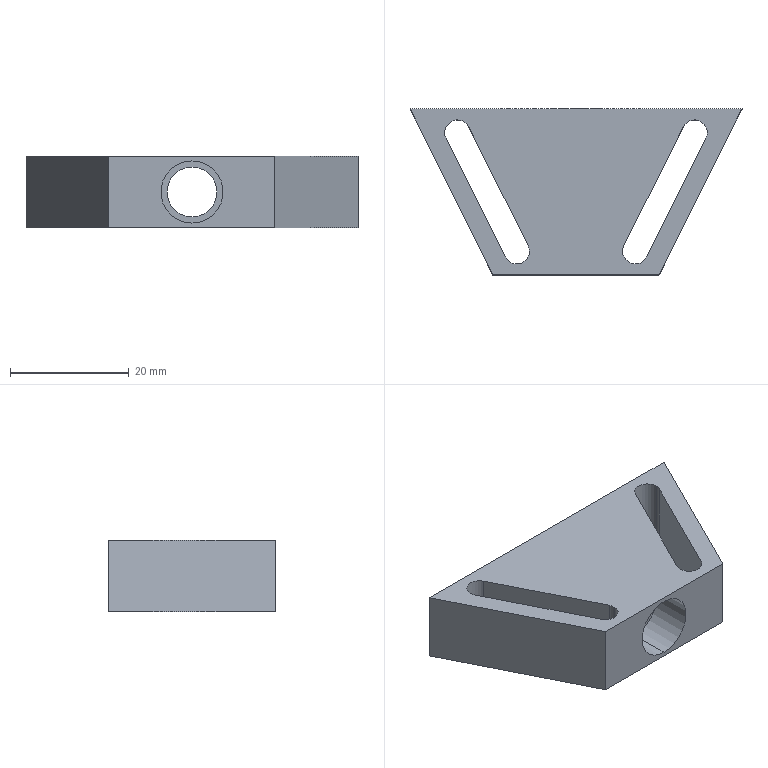Part | SolidWorks | features BaseBody 1 | 1 solid | 21 faces | box 56 x 28 x 12 mm | volume 9686 mm3 | plane 11 | cylinder 10 | commonest cylinder face diameters 4.3 x6 8.4 x2 10.5 x2
STEP:
#1=CARTESIAN_POINT('',(18.077,10.962,-6.));
#2=VERTEX_POINT('',#1);
#3=CARTESIAN_POINT('',(22.15,10.,-6.));
#4=VERTEX_POINT('',#3);
#5=CARTESIAN_POINT('',(20.,10.,-6.));
#6=DIRECTION('',(0.,0.,-1.));
#7=DIRECTION('',(1.,0.,0.));
#8=AXIS2_PLACEMENT_3D('',#5,#6,#7);
#9=CIRCLE('',#8,2.15);
#10=EDGE_CURVE('',#2,#4,#9,.T.);
#11=ORIENTED_EDGE('',*,*,#10,.T.);
#12=CARTESIAN_POINT('',(22.15,10.,6.));
#13=VERTEX_POINT('',#12);
#14=CARTESIAN_POINT('',(22.15,10.,-7.));
#15=DIRECTION('',(0.,0.,1.));
#16=VECTOR('',#15,1000.);
#17=LINE('',#14,#16);
#18=EDGE_CURVE('',#4,#13,#17,.T.);
#19=ORIENTED_EDGE('',*,*,#18,.T.);
#20=CARTESIAN_POINT('',(18.077,10.962,6.));
#21=VERTEX_POINT('',#20);
#22=CARTESIAN_POINT('',(20.,10.,6.));
#23=DIRECTION('',(0.,0.,-1.));
#24=DIRECTION('',(1.,0.,0.));
#25=AXIS2_PLACEMENT_3D('',#22,#23,#24);
#26=CIRCLE('',#25,2.15);
#27=EDGE_CURVE('',#21,#13,#26,.T.);
#28=ORIENTED_EDGE('',*,*,#27,.F.);
#29=CARTESIAN_POINT('',(18.077,10.962,-7.));
#30=DIRECTION('',(0.,0.,1.));
#31=VECTOR('',#30,1000.);
#32=LINE('',#29,#31);
#33=EDGE_CURVE('',#2,#21,#32,.T.);
#34=ORIENTED_EDGE('',*,*,#33,.F.);
#35=EDGE_LOOP('',(#11,#19,#28,#34));
#36=FACE_OUTER_BOUND('',#35,.T.);
#37=CARTESIAN_POINT('',(20.,10.,-7.));
#38=DIRECTION('',(0.,0.,1.));
#39=DIRECTION('',(1.,0.,0.));
#40=AXIS2_PLACEMENT_3D('',#37,#38,#39);
#41=CYLINDRICAL_SURFACE('',#40,2.15);
#42=ADVANCED_FACE('',(#36),#41,.F.);
#43=CARTESIAN_POINT('',(-8.077,-9.038,-6.));
#44=VERTEX_POINT('',#43);
#45=CARTESIAN_POINT('',(-7.85,-10.,-6.));
#46=VERTEX_POINT('',#45);
#47=CARTESIAN_POINT('',(-10.,-10.,-6.));
#48=DIRECTION('',(0.,0.,-1.));
#49=DIRECTION('',(1.,0.,0.));
#50=AXIS2_PLACEMENT_3D('',#47,#48,#49);
#51=CIRCLE('',#50,2.15);
#52=EDGE_CURVE('',#44,#46,#51,.T.);
#53=ORIENTED_EDGE('',*,*,#52,.T.);
#54=CARTESIAN_POINT('',(-7.85,-10.,6.));
#55=VERTEX_POINT('',#54);
#56=CARTESIAN_POINT('',(-7.85,-10.,-7.));
#57=DIRECTION('',(0.,0.,1.));
#58=VECTOR('',#57,1000.);
#59=LINE('',#56,#58);
#60=EDGE_CURVE('',#46,#55,#59,.T.);
#61=ORIENTED_EDGE('',*,*,#60,.T.);
#62=CARTESIAN_POINT('',(-8.077,-9.038,6.));
#63=VERTEX_POINT('',#62);
#64=CARTESIAN_POINT('',(-10.,-10.,6.));
#65=DIRECTION('',(0.,0.,-1.));
#66=DIRECTION('',(1.,0.,0.));
#67=AXIS2_PLACEMENT_3D('',#64,#65,#66);
#68=CIRCLE('',#67,2.15);
#69=EDGE_CURVE('',#63,#55,#68,.T.);
#70=ORIENTED_EDGE('',*,*,#69,.F.);
#71=CARTESIAN_POINT('',(-8.077,-9.038,-7.));
#72=DIRECTION('',(0.,0.,-1.));
#73=VECTOR('',#72,1000.);
#74=LINE('',#71,#73);
#75=EDGE_CURVE('',#63,#44,#74,.T.);
#76=ORIENTED_EDGE('',*,*,#75,.T.);
#77=EDGE_LOOP('',(#53,#61,#70,#76));
#78=FACE_OUTER_BOUND('',#77,.T.);
#79=CARTESIAN_POINT('',(-10.,-10.,-7.));
#80=DIRECTION('',(0.,0.,1.));
#81=DIRECTION('',(1.,0.,0.));
#82=AXIS2_PLACEMENT_3D('',#79,#80,#81);
#83=CYLINDRICAL_SURFACE('',#82,2.15);
#84=ADVANCED_FACE('',(#78),#83,.F.);
#85=CARTESIAN_POINT('',(0.,-7.,-4.2));
#86=VERTEX_POINT('',#85);
#87=CARTESIAN_POINT('',(0.,-7.,4.2));
#88=VERTEX_POINT('',#87);
#89=CARTESIAN_POINT('',(0.,-7.,0.));
#90=DIRECTION('',(0.,1.,0.));
#91=DIRECTION('',(0.,0.,1.));
#92=AXIS2_PLACEMENT_3D('',#89,#90,#91);
#93=CIRCLE('',#92,4.2);
#94=EDGE_CURVE('',#86,#88,#93,.T.);
#95=ORIENTED_EDGE('',*,*,#94,.F.);
#96=CARTESIAN_POINT('',(0.,14.,-4.2));
#97=VERTEX_POINT('',#96);
#98=CARTESIAN_POINT('',(0.,-16.,-4.2));
#99=DIRECTION('',(0.,1.,0.));
#100=VECTOR('',#99,1000.);
#101=LINE('',#98,#100);
#102=EDGE_CURVE('',#86,#97,#101,.T.);
#103=ORIENTED_EDGE('',*,*,#102,.T.);
#104=CARTESIAN_POINT('',(0.,14.,4.2));
#105=VERTEX_POINT('',#104);
#106=CARTESIAN_POINT('',(0.,14.,0.));
#107=DIRECTION('',(0.,1.,0.));
#108=DIRECTION('',(0.,0.,1.));
#109=AXIS2_PLACEMENT_3D('',#106,#107,#108);
#110=CIRCLE('',#109,4.2);
#111=EDGE_CURVE('',#97,#105,#110,.T.);
#112=ORIENTED_EDGE('',*,*,#111,.T.);
#113=CARTESIAN_POINT('',(0.,-16.,4.2));
#114=DIRECTION('',(0.,1.,0.));
#115=VECTOR('',#114,1000.);
#116=LINE('',#113,#115);
#117=EDGE_CURVE('',#88,#105,#116,.T.);
#118=ORIENTED_EDGE('',*,*,#117,.F.);
#119=EDGE_LOOP('',(#95,#103,#112,#118));
#120=FACE_OUTER_BOUND('',#119,.T.);
#121=CARTESIAN_POINT('',(0.,-16.,0.));
#122=DIRECTION('',(0.,1.,0.));
#123=DIRECTION('',(0.,0.,1.));
#124=AXIS2_PLACEMENT_3D('',#121,#122,#123);
#125=CYLINDRICAL_SURFACE('',#124,4.2);
#126=ADVANCED_FACE('',(#120),#125,.F.);
#127=CARTESIAN_POINT('',(0.,-14.,5.25));
#128=VERTEX_POINT('',#127);
#129=CARTESIAN_POINT('',(0.,-14.,-5.25));
#130=VERTEX_POINT('',#129);
#131=CARTESIAN_POINT('',(0.,-14.,0.));
#132=DIRECTION('',(0.,-1.,0.));
#133=DIRECTION('',(0.,0.,1.));
#134=AXIS2_PLACEMENT_3D('',#131,#132,#133);
#135=CIRCLE('',#134,5.25);
#136=EDGE_CURVE('',#128,#130,#135,.T.);
#137=ORIENTED_EDGE('',*,*,#136,.T.);
#138=CARTESIAN_POINT('',(0.,-7.,-5.25));
#139=VERTEX_POINT('',#138);
#140=CARTESIAN_POINT('',(0.,-14.,-5.25));
#141=DIRECTION('',(0.,1.,0.));
#142=VECTOR('',#141,1000.);
#143=LINE('',#140,#142);
#144=EDGE_CURVE('',#130,#139,#143,.T.);
#145=ORIENTED_EDGE('',*,*,#144,.T.);
#146=CARTESIAN_POINT('',(0.,-7.,5.25));
#147=VERTEX_POINT('',#146);
#148=CARTESIAN_POINT('',(0.,-7.,0.));
#149=DIRECTION('',(0.,-1.,0.));
#150=DIRECTION('',(0.,0.,1.));
#151=AXIS2_PLACEMENT_3D('',#148,#149,#150);
#152=CIRCLE('',#151,5.25);
#153=EDGE_CURVE('',#147,#139,#152,.T.);
#154=ORIENTED_EDGE('',*,*,#153,.F.);
#155=CARTESIAN_POINT('',(0.,-14.,5.25));
#156=DIRECTION('',(0.,1.,0.));
#157=VECTOR('',#156,1000.);
#158=LINE('',#155,#157);
#159=EDGE_CURVE('',#128,#147,#158,.T.);
#160=ORIENTED_EDGE('',*,*,#159,.F.);
#161=EDGE_LOOP('',(#137,#145,#154,#160));
#162=FACE_OUTER_BOUND('',#161,.T.);
#163=CARTESIAN_POINT('',(0.,-14.,0.));
#164=DIRECTION('',(0.,1.,0.));
#165=DIRECTION('',(0.,0.,1.));
#166=AXIS2_PLACEMENT_3D('',#163,#164,#165);
#167=CYLINDRICAL_SURFACE('',#166,5.25);
#168=ADVANCED_FACE('',(#162),#167,.F.);
#169=ORIENTED_EDGE('',*,*,#10,.F.);
#170=CARTESIAN_POINT('',(8.077,-9.038,-6.));
#171=VERTEX_POINT('',#170);
#172=CARTESIAN_POINT('',(8.077,-9.038,-6.));
#173=DIRECTION('',(0.4472,0.8944,0.));
#174=VECTOR('',#173,1000.);
#175=LINE('',#172,#174);
#176=EDGE_CURVE('',#171,#2,#175,.T.);
#177=ORIENTED_EDGE('',*,*,#176,.F.);
#178=CARTESIAN_POINT('',(11.923,-10.962,-6.));
#179=VERTEX_POINT('',#178);
#180=CARTESIAN_POINT('',(10.,-10.,-6.));
#181=DIRECTION('',(0.,0.,-1.));
#182=DIRECTION('',(1.,0.,0.));
#183=AXIS2_PLACEMENT_3D('',#180,#181,#182);
#184=CIRCLE('',#183,2.15);
#185=EDGE_CURVE('',#179,#171,#184,.T.);
#186=ORIENTED_EDGE('',*,*,#185,.F.);
#187=CARTESIAN_POINT('',(21.923,9.038,-6.));
#188=VERTEX_POINT('',#187);
#189=CARTESIAN_POINT('',(21.923,9.038,-6.));
#190=DIRECTION('',(-0.4472,-0.8944,0.));
#191=VECTOR('',#190,1000.);
#192=LINE('',#189,#191);
#193=EDGE_CURVE('',#188,#179,#192,.T.);
#194=ORIENTED_EDGE('',*,*,#193,.F.);
#195=CARTESIAN_POINT('',(20.,10.,-6.));
#196=DIRECTION('',(0.,0.,-1.));
#197=DIRECTION('',(1.,0.,0.));
#198=AXIS2_PLACEMENT_3D('',#195,#196,#197);
#199=CIRCLE('',#198,2.15);
#200=EDGE_CURVE('',#4,#188,#199,.T.);
#201=ORIENTED_EDGE('',*,*,#200,.F.);
#202=EDGE_LOOP('',(#169,#177,#186,#194,#201));
#203=FACE_BOUND('',#202,.T.);
#204=CARTESIAN_POINT('',(-21.923,9.038,-6.));
#205=VERTEX_POINT('',#204);
#206=CARTESIAN_POINT('',(-18.077,10.962,-6.));
#207=VERTEX_POINT('',#206);
#208=CARTESIAN_POINT('',(-20.,10.,-6.));
#209=DIRECTION('',(0.,0.,-1.));
#210=DIRECTION('',(1.,0.,0.));
#211=AXIS2_PLACEMENT_3D('',#208,#209,#210);
#212=CIRCLE('',#211,2.15);
#213=EDGE_CURVE('',#205,#207,#212,.T.);
#214=ORIENTED_EDGE('',*,*,#213,.F.);
#215=CARTESIAN_POINT('',(-11.923,-10.962,-6.));
#216=VERTEX_POINT('',#215);
#217=CARTESIAN_POINT('',(-11.923,-10.962,-6.));
#218=DIRECTION('',(-0.4472,0.8944,0.));
#219=VECTOR('',#218,1000.);
#220=LINE('',#217,#219);
#221=EDGE_CURVE('',#216,#205,#220,.T.);
#222=ORIENTED_EDGE('',*,*,#221,.F.);
#223=CARTESIAN_POINT('',(-10.,-10.,-6.));
#224=DIRECTION('',(0.,0.,-1.));
#225=DIRECTION('',(1.,0.,0.));
#226=AXIS2_PLACEMENT_3D('',#223,#224,#225);
#227=CIRCLE('',#226,2.15);
#228=EDGE_CURVE('',#46,#216,#227,.T.);
#229=ORIENTED_EDGE('',*,*,#228,.F.);
#230=ORIENTED_EDGE('',*,*,#52,.F.);
#231=CARTESIAN_POINT('',(-18.077,10.962,-6.));
#232=DIRECTION('',(0.4472,-0.8944,0.));
#233=VECTOR('',#232,1000.);
#234=LINE('',#231,#233);
#235=EDGE_CURVE('',#207,#44,#234,.T.);
#236=ORIENTED_EDGE('',*,*,#235,.F.);
#237=EDGE_LOOP('',(#214,#222,#229,#230,#236));
#238=FACE_BOUND('',#237,.T.);
#239=CARTESIAN_POINT('',(28.,14.,-6.));
#240=VERTEX_POINT('',#239);
#241=CARTESIAN_POINT('',(-28.,14.,-6.));
#242=VERTEX_POINT('',#241);
#243=CARTESIAN_POINT('',(0.,14.,-6.));
#244=DIRECTION('',(-1.,0.,0.));
#245=VECTOR('',#244,1000.);
#246=LINE('',#243,#245);
#247=EDGE_CURVE('',#240,#242,#246,.T.);
#248=ORIENTED_EDGE('',*,*,#247,.F.);
#249=CARTESIAN_POINT('',(14.,-14.,-6.));
#250=VERTEX_POINT('',#249);
#251=CARTESIAN_POINT('',(14.,-14.,-6.));
#252=DIRECTION('',(0.4472,0.8944,0.));
#253=VECTOR('',#252,1000.);
#254=LINE('',#251,#253);
#255=EDGE_CURVE('',#250,#240,#254,.T.);
#256=ORIENTED_EDGE('',*,*,#255,.F.);
#257=CARTESIAN_POINT('',(-14.,-14.,-6.));
#258=VERTEX_POINT('',#257);
#259=CARTESIAN_POINT('',(0.,-14.,-6.));
#260=DIRECTION('',(1.,0.,0.));
#261=VECTOR('',#260,1000.);
#262=LINE('',#259,#261);
#263=EDGE_CURVE('',#258,#250,#262,.T.);
#264=ORIENTED_EDGE('',*,*,#263,.F.);
#265=CARTESIAN_POINT('',(-28.,14.,-6.));
#266=DIRECTION('',(0.4472,-0.8944,0.));
#267=VECTOR('',#266,1000.);
#268=LINE('',#265,#267);
#269=EDGE_CURVE('',#242,#258,#268,.T.);
#270=ORIENTED_EDGE('',*,*,#269,.F.);
#271=EDGE_LOOP('',(#248,#256,#264,#270));
#272=FACE_OUTER_BOUND('',#271,.T.);
#273=CARTESIAN_POINT('',(0.,2.674,-6.));
#274=DIRECTION('',(0.,0.,1.));
#275=DIRECTION('',(1.,0.,0.));
#276=AXIS2_PLACEMENT_3D('',#273,#274,#275);
#277=PLANE('',#276);
#278=ADVANCED_FACE('',(#203,#238,#272),#277,.F.);
#279=CARTESIAN_POINT('',(21.923,9.038,6.));
#280=VERTEX_POINT('',#279);
#281=CARTESIAN_POINT('',(21.923,9.038,-7.));
#282=DIRECTION('',(0.,0.,1.));
#283=VECTOR('',#282,1000.);
#284=LINE('',#281,#283);
#285=EDGE_CURVE('',#188,#280,#284,.T.);
#286=ORIENTED_EDGE('',*,*,#285,.F.);
#287=ORIENTED_EDGE('',*,*,#193,.T.);
#288=CARTESIAN_POINT('',(11.923,-10.962,6.));
#289=VERTEX_POINT('',#288);
#290=CARTESIAN_POINT('',(11.923,-10.962,-7.));
#291=DIRECTION('',(0.,0.,-1.));
#292=VECTOR('',#291,1000.);
#293=LINE('',#290,#292);
#294=EDGE_CURVE('',#289,#179,#293,.T.);
#295=ORIENTED_EDGE('',*,*,#294,.F.);
#296=CARTESIAN_POINT('',(11.923,-10.962,6.));
#297=DIRECTION('',(-0.4472,-0.8944,0.));
#298=VECTOR('',#297,1000.);
#299=LINE('',#296,#298);
#300=EDGE_CURVE('',#280,#289,#299,.T.);
#301=ORIENTED_EDGE('',*,*,#300,.F.);
#302=EDGE_LOOP('',(#286,#287,#295,#301));
#303=FACE_OUTER_BOUND('',#302,.T.);
#304=CARTESIAN_POINT('',(11.923,-10.962,-7.));
#305=DIRECTION('',(0.8944,-0.4472,0.));
#306=DIRECTION('',(0.4472,0.8944,0.));
#307=AXIS2_PLACEMENT_3D('',#304,#305,#306);
#308=PLANE('',#307);
#309=ADVANCED_FACE('',(#303),#308,.F.);
#310=ORIENTED_EDGE('',*,*,#18,.F.);
#311=ORIENTED_EDGE('',*,*,#200,.T.);
#312=ORIENTED_EDGE('',*,*,#285,.T.);
#313=CARTESIAN_POINT('',(20.,10.,6.));
#314=DIRECTION('',(0.,0.,-1.));
#315=DIRECTION('',(1.,0.,0.));
#316=AXIS2_PLACEMENT_3D('',#313,#314,#315);
#317=CIRCLE('',#316,2.15);
#318=EDGE_CURVE('',#13,#280,#317,.T.);
#319=ORIENTED_EDGE('',*,*,#318,.F.);
#320=EDGE_LOOP('',(#310,#311,#312,#319));
#321=FACE_OUTER_BOUND('',#320,.T.);
#322=CARTESIAN_POINT('',(20.,10.,-7.));
#323=DIRECTION('',(0.,0.,1.));
#324=DIRECTION('',(1.,0.,0.));
#325=AXIS2_PLACEMENT_3D('',#322,#323,#324);
#326=CYLINDRICAL_SURFACE('',#325,2.15);
#327=ADVANCED_FACE('',(#321),#326,.F.);
#328=ORIENTED_EDGE('',*,*,#33,.T.);
#329=CARTESIAN_POINT('',(8.077,-9.038,6.));
#330=VERTEX_POINT('',#329);
#331=CARTESIAN_POINT('',(8.077,-9.038,6.));
#332=DIRECTION('',(-0.4472,-0.8944,0.));
#333=VECTOR('',#332,1000.);
#334=LINE('',#331,#333);
#335=EDGE_CURVE('',#21,#330,#334,.T.);
#336=ORIENTED_EDGE('',*,*,#335,.T.);
#337=CARTESIAN_POINT('',(8.077,-9.038,-7.));
#338=DIRECTION('',(0.,0.,-1.));
#339=VECTOR('',#338,1000.);
#340=LINE('',#337,#339);
#341=EDGE_CURVE('',#330,#171,#340,.T.);
#342=ORIENTED_EDGE('',*,*,#341,.T.);
#343=ORIENTED_EDGE('',*,*,#176,.T.);
#344=EDGE_LOOP('',(#328,#336,#342,#343));
#345=FACE_OUTER_BOUND('',#344,.T.);
#346=CARTESIAN_POINT('',(8.077,-9.038,-7.));
#347=DIRECTION('',(0.8944,-0.4472,0.));
#348=DIRECTION('',(0.4472,0.8944,0.));
#349=AXIS2_PLACEMENT_3D('',#346,#347,#348);
#350=PLANE('',#349);
#351=ADVANCED_FACE('',(#345),#350,.T.);
#352=ORIENTED_EDGE('',*,*,#185,.T.);
#353=ORIENTED_EDGE('',*,*,#341,.F.);
#354=CARTESIAN_POINT('',(10.,-10.,6.));
#355=DIRECTION('',(0.,0.,-1.));
#356=DIRECTION('',(1.,0.,0.));
#357=AXIS2_PLACEMENT_3D('',#354,#355,#356);
#358=CIRCLE('',#357,2.15);
#359=EDGE_CURVE('',#289,#330,#358,.T.);
#360=ORIENTED_EDGE('',*,*,#359,.F.);
#361=ORIENTED_EDGE('',*,*,#294,.T.);
#362=EDGE_LOOP('',(#352,#353,#360,#361));
#363=FACE_OUTER_BOUND('',#362,.T.);
#364=CARTESIAN_POINT('',(10.,-10.,-7.));
#365=DIRECTION('',(0.,0.,1.));
#366=DIRECTION('',(1.,0.,0.));
#367=AXIS2_PLACEMENT_3D('',#364,#365,#366);
#368=CYLINDRICAL_SURFACE('',#367,2.15);
#369=ADVANCED_FACE('',(#363),#368,.F.);
#370=CARTESIAN_POINT('',(-18.077,10.962,6.));
#371=VERTEX_POINT('',#370);
#372=CARTESIAN_POINT('',(-18.077,10.962,-7.));
#373=DIRECTION('',(0.,0.,1.));
#374=VECTOR('',#373,1000.);
#375=LINE('',#372,#374);
#376=EDGE_CURVE('',#207,#371,#375,.T.);
#377=ORIENTED_EDGE('',*,*,#376,.F.);
#378=ORIENTED_EDGE('',*,*,#235,.T.);
#379=ORIENTED_EDGE('',*,*,#75,.F.);
#380=CARTESIAN_POINT('',(-8.077,-9.038,6.));
#381=DIRECTION('',(0.4472,-0.8944,0.));
#382=VECTOR('',#381,1000.);
#383=LINE('',#380,#382);
#384=EDGE_CURVE('',#371,#63,#383,.T.);
#385=ORIENTED_EDGE('',*,*,#384,.F.);
#386=EDGE_LOOP('',(#377,#378,#379,#385));
#387=FACE_OUTER_BOUND('',#386,.T.);
#388=CARTESIAN_POINT('',(-8.077,-9.038,-7.));
#389=DIRECTION('',(0.8944,0.4472,0.));
#390=DIRECTION('',(-0.4472,0.8944,0.));
#391=AXIS2_PLACEMENT_3D('',#388,#389,#390);
#392=PLANE('',#391);
#393=ADVANCED_FACE('',(#387),#392,.F.);
#394=ORIENTED_EDGE('',*,*,#213,.T.);
#395=ORIENTED_EDGE('',*,*,#376,.T.);
#396=CARTESIAN_POINT('',(-21.923,9.038,6.));
#397=VERTEX_POINT('',#396);
#398=CARTESIAN_POINT('',(-20.,10.,6.));
#399=DIRECTION('',(0.,0.,-1.));
#400=DIRECTION('',(1.,0.,0.));
#401=AXIS2_PLACEMENT_3D('',#398,#399,#400);
#402=CIRCLE('',#401,2.15);
#403=EDGE_CURVE('',#397,#371,#402,.T.);
#404=ORIENTED_EDGE('',*,*,#403,.F.);
#405=CARTESIAN_POINT('',(-21.923,9.038,-7.));
#406=DIRECTION('',(0.,0.,1.));
#407=VECTOR('',#406,1000.);
#408=LINE('',#405,#407);
#409=EDGE_CURVE('',#205,#397,#408,.T.);
#410=ORIENTED_EDGE('',*,*,#409,.F.);
#411=EDGE_LOOP('',(#394,#395,#404,#410));
#412=FACE_OUTER_BOUND('',#411,.T.);
#413=CARTESIAN_POINT('',(-20.,10.,-7.));
#414=DIRECTION('',(0.,0.,1.));
#415=DIRECTION('',(1.,0.,0.));
#416=AXIS2_PLACEMENT_3D('',#413,#414,#415);
#417=CYLINDRICAL_SURFACE('',#416,2.15);
#418=ADVANCED_FACE('',(#412),#417,.F.);
#419=ORIENTED_EDGE('',*,*,#409,.T.);
#420=CARTESIAN_POINT('',(-11.923,-10.962,6.));
#421=VERTEX_POINT('',#420);
#422=CARTESIAN_POINT('',(-11.923,-10.962,6.));
#423=DIRECTION('',(0.4472,-0.8944,0.));
#424=VECTOR('',#423,1000.);
#425=LINE('',#422,#424);
#426=EDGE_CURVE('',#397,#421,#425,.T.);
#427=ORIENTED_EDGE('',*,*,#426,.T.);
#428=CARTESIAN_POINT('',(-11.923,-10.962,-7.));
#429=DIRECTION('',(0.,0.,-1.));
#430=VECTOR('',#429,1000.);
#431=LINE('',#428,#430);
#432=EDGE_CURVE('',#421,#216,#431,.T.);
#433=ORIENTED_EDGE('',*,*,#432,.T.);
#434=ORIENTED_EDGE('',*,*,#221,.T.);
#435=EDGE_LOOP('',(#419,#427,#433,#434));
#436=FACE_OUTER_BOUND('',#435,.T.);
#437=CARTESIAN_POINT('',(-11.923,-10.962,-7.));
#438=DIRECTION('',(0.8944,0.4472,0.));
#439=DIRECTION('',(-0.4472,0.8944,0.));
#440=AXIS2_PLACEMENT_3D('',#437,#438,#439);
#441=PLANE('',#440);
#442=ADVANCED_FACE('',(#436),#441,.T.);
#443=ORIENTED_EDGE('',*,*,#60,.F.);
#444=ORIENTED_EDGE('',*,*,#228,.T.);
#445=ORIENTED_EDGE('',*,*,#432,.F.);
#446=CARTESIAN_POINT('',(-10.,-10.,6.));
#447=DIRECTION('',(0.,0.,-1.));
#448=DIRECTION('',(1.,0.,0.));
#449=AXIS2_PLACEMENT_3D('',#446,#447,#448);
#450=CIRCLE('',#449,2.15);
#451=EDGE_CURVE('',#55,#421,#450,.T.);
#452=ORIENTED_EDGE('',*,*,#451,.F.);
#453=EDGE_LOOP('',(#443,#444,#445,#452));
#454=FACE_OUTER_BOUND('',#453,.T.);
#455=CARTESIAN_POINT('',(-10.,-10.,-7.));
#456=DIRECTION('',(0.,0.,1.));
#457=DIRECTION('',(1.,0.,0.));
#458=AXIS2_PLACEMENT_3D('',#455,#456,#457);
#459=CYLINDRICAL_SURFACE('',#458,2.15);
#460=ADVANCED_FACE('',(#454),#459,.F.);
#461=CARTESIAN_POINT('',(-14.,-14.,6.));
#462=VERTEX_POINT('',#461);
#463=CARTESIAN_POINT('',(-14.,-14.,-6.));
#464=DIRECTION('',(0.,0.,-1.));
#465=VECTOR('',#464,1000.);
#466=LINE('',#463,#465);
#467=EDGE_CURVE('',#462,#258,#466,.T.);
#468=ORIENTED_EDGE('',*,*,#467,.F.);
#469=CARTESIAN_POINT('',(-28.,14.,6.));
#470=VERTEX_POINT('',#469);
#471=CARTESIAN_POINT('',(-28.,14.,6.));
#472=DIRECTION('',(0.4472,-0.8944,0.));
#473=VECTOR('',#472,1000.);
#474=LINE('',#471,#473);
#475=EDGE_CURVE('',#470,#462,#474,.T.);
#476=ORIENTED_EDGE('',*,*,#475,.F.);
#477=CARTESIAN_POINT('',(-28.,14.,-6.));
#478=DIRECTION('',(0.,0.,1.));
#479=VECTOR('',#478,1000.);
#480=LINE('',#477,#479);
#481=EDGE_CURVE('',#242,#470,#480,.T.);
#482=ORIENTED_EDGE('',*,*,#481,.F.);
#483=ORIENTED_EDGE('',*,*,#269,.T.);
#484=EDGE_LOOP('',(#468,#476,#482,#483));
#485=FACE_OUTER_BOUND('',#484,.T.);
#486=CARTESIAN_POINT('',(-28.,14.,-6.));
#487=DIRECTION('',(0.8944,0.4472,0.));
#488=DIRECTION('',(-0.4472,0.8944,0.));
#489=AXIS2_PLACEMENT_3D('',#486,#487,#488);
#490=PLANE('',#489);
#491=ADVANCED_FACE('',(#485),#490,.F.);
#492=CARTESIAN_POINT('',(0.,14.,0.));
#493=DIRECTION('',(0.,1.,0.));
#494=DIRECTION('',(0.,0.,1.));
#495=AXIS2_PLACEMENT_3D('',#492,#493,#494);
#496=CIRCLE('',#495,4.2);
#497=EDGE_CURVE('',#105,#97,#496,.T.);
#498=ORIENTED_EDGE('',*,*,#497,.F.);
#499=ORIENTED_EDGE('',*,*,#111,.F.);
#500=EDGE_LOOP('',(#498,#499));
#501=FACE_BOUND('',#500,.T.);
#502=ORIENTED_EDGE('',*,*,#481,.T.);
#503=CARTESIAN_POINT('',(28.,14.,6.));
#504=VERTEX_POINT('',#503);
#505=CARTESIAN_POINT('',(28.,14.,6.));
#506=DIRECTION('',(-1.,0.,0.));
#507=VECTOR('',#506,1000.);
#508=LINE('',#505,#507);
#509=EDGE_CURVE('',#504,#470,#508,.T.);
#510=ORIENTED_EDGE('',*,*,#509,.F.);
#511=CARTESIAN_POINT('',(28.,14.,-6.));
#512=DIRECTION('',(0.,0.,1.));
#513=VECTOR('',#512,1000.);
#514=LINE('',#511,#513);
#515=EDGE_CURVE('',#240,#504,#514,.T.);
#516=ORIENTED_EDGE('',*,*,#515,.F.);
#517=ORIENTED_EDGE('',*,*,#247,.T.);
#518=EDGE_LOOP('',(#502,#510,#516,#517));
#519=FACE_OUTER_BOUND('',#518,.T.);
#520=CARTESIAN_POINT('',(28.,14.,-6.));
#521=DIRECTION('',(0.,-1.,0.));
#522=DIRECTION('',(0.,0.,-1.));
#523=AXIS2_PLACEMENT_3D('',#520,#521,#522);
#524=PLANE('',#523);
#525=ADVANCED_FACE('',(#501,#519),#524,.F.);
#526=ORIENTED_EDGE('',*,*,#515,.T.);
#527=CARTESIAN_POINT('',(14.,-14.,6.));
#528=VERTEX_POINT('',#527);
#529=CARTESIAN_POINT('',(14.,-14.,6.));
#530=DIRECTION('',(0.4472,0.8944,0.));
#531=VECTOR('',#530,1000.);
#532=LINE('',#529,#531);
#533=EDGE_CURVE('',#528,#504,#532,.T.);
#534=ORIENTED_EDGE('',*,*,#533,.F.);
#535=CARTESIAN_POINT('',(14.,-14.,-6.));
#536=DIRECTION('',(0.,0.,1.));
#537=VECTOR('',#536,1000.);
#538=LINE('',#535,#537);
#539=EDGE_CURVE('',#250,#528,#538,.T.);
#540=ORIENTED_EDGE('',*,*,#539,.F.);
#541=ORIENTED_EDGE('',*,*,#255,.T.);
#542=EDGE_LOOP('',(#526,#534,#540,#541));
#543=FACE_OUTER_BOUND('',#542,.T.);
#544=CARTESIAN_POINT('',(14.,-14.,-6.));
#545=DIRECTION('',(-0.8944,0.4472,0.));
#546=DIRECTION('',(-0.4472,-0.8944,0.));
#547=AXIS2_PLACEMENT_3D('',#544,#545,#546);
#548=PLANE('',#547);
#549=ADVANCED_FACE('',(#543),#548,.F.);
#550=ORIENTED_EDGE('',*,*,#136,.F.);
#551=CARTESIAN_POINT('',(0.,-14.,0.));
#552=DIRECTION('',(0.,-1.,0.));
#553=DIRECTION('',(0.,0.,1.));
#554=AXIS2_PLACEMENT_3D('',#551,#552,#553);
#555=CIRCLE('',#554,5.25);
#556=EDGE_CURVE('',#130,#128,#555,.T.);
#557=ORIENTED_EDGE('',*,*,#556,.F.);
#558=EDGE_LOOP('',(#550,#557));
#559=FACE_BOUND('',#558,.T.);
#560=ORIENTED_EDGE('',*,*,#539,.T.);
#561=CARTESIAN_POINT('',(-14.,-14.,6.));
#562=DIRECTION('',(1.,0.,0.));
#563=VECTOR('',#562,1000.);
#564=LINE('',#561,#563);
#565=EDGE_CURVE('',#462,#528,#564,.T.);
#566=ORIENTED_EDGE('',*,*,#565,.F.);
#567=ORIENTED_EDGE('',*,*,#467,.T.);
#568=ORIENTED_EDGE('',*,*,#263,.T.);
#569=EDGE_LOOP('',(#560,#566,#567,#568));
#570=FACE_OUTER_BOUND('',#569,.T.);
#571=CARTESIAN_POINT('',(-14.,-14.,-6.));
#572=DIRECTION('',(0.,1.,0.));
#573=DIRECTION('',(0.,0.,1.));
#574=AXIS2_PLACEMENT_3D('',#571,#572,#573);
#575=PLANE('',#574);
#576=ADVANCED_FACE('',(#559,#570),#575,.F.);
#577=ORIENTED_EDGE('',*,*,#27,.T.);
#578=ORIENTED_EDGE('',*,*,#318,.T.);
#579=ORIENTED_EDGE('',*,*,#300,.T.);
#580=ORIENTED_EDGE('',*,*,#359,.T.);
#581=ORIENTED_EDGE('',*,*,#335,.F.);
#582=EDGE_LOOP('',(#577,#578,#579,#580,#581));
#583=FACE_BOUND('',#582,.T.);
#584=ORIENTED_EDGE('',*,*,#403,.T.);
#585=ORIENTED_EDGE('',*,*,#384,.T.);
#586=ORIENTED_EDGE('',*,*,#69,.T.);
#587=ORIENTED_EDGE('',*,*,#451,.T.);
#588=ORIENTED_EDGE('',*,*,#426,.F.);
#589=EDGE_LOOP('',(#584,#585,#586,#587,#588));
#590=FACE_BOUND('',#589,.T.);
#591=ORIENTED_EDGE('',*,*,#509,.T.);
#592=ORIENTED_EDGE('',*,*,#475,.T.);
#593=ORIENTED_EDGE('',*,*,#565,.T.);
#594=ORIENTED_EDGE('',*,*,#533,.T.);
#595=EDGE_LOOP('',(#591,#592,#593,#594));
#596=FACE_OUTER_BOUND('',#595,.T.);
#597=CARTESIAN_POINT('',(0.,2.674,6.));
#598=DIRECTION('',(0.,0.,1.));
#599=DIRECTION('',(1.,0.,0.));
#600=AXIS2_PLACEMENT_3D('',#597,#598,#599);
#601=PLANE('',#600);
#602=ADVANCED_FACE('',(#583,#590,#596),#601,.T.);
#603=ORIENTED_EDGE('',*,*,#102,.F.);
#604=CARTESIAN_POINT('',(0.,-7.,0.));
#605=DIRECTION('',(0.,1.,0.));
#606=DIRECTION('',(0.,0.,1.));
#607=AXIS2_PLACEMENT_3D('',#604,#605,#606);
#608=CIRCLE('',#607,4.2);
#609=EDGE_CURVE('',#88,#86,#608,.T.);
#610=ORIENTED_EDGE('',*,*,#609,.F.);
#611=ORIENTED_EDGE('',*,*,#117,.T.);
#612=ORIENTED_EDGE('',*,*,#497,.T.);
#613=EDGE_LOOP('',(#603,#610,#611,#612));
#614=FACE_OUTER_BOUND('',#613,.T.);
#615=CARTESIAN_POINT('',(0.,-16.,0.));
#616=DIRECTION('',(0.,1.,0.));
#617=DIRECTION('',(0.,0.,1.));
#618=AXIS2_PLACEMENT_3D('',#615,#616,#617);
#619=CYLINDRICAL_SURFACE('',#618,4.2);
#620=ADVANCED_FACE('',(#614),#619,.F.);
#621=ORIENTED_EDGE('',*,*,#144,.F.);
#622=ORIENTED_EDGE('',*,*,#556,.T.);
#623=ORIENTED_EDGE('',*,*,#159,.T.);
#624=CARTESIAN_POINT('',(0.,-7.,0.));
#625=DIRECTION('',(0.,-1.,0.));
#626=DIRECTION('',(0.,0.,1.));
#627=AXIS2_PLACEMENT_3D('',#624,#625,#626);
#628=CIRCLE('',#627,5.25);
#629=EDGE_CURVE('',#139,#147,#628,.T.);
#630=ORIENTED_EDGE('',*,*,#629,.F.);
#631=EDGE_LOOP('',(#621,#622,#623,#630));
#632=FACE_OUTER_BOUND('',#631,.T.);
#633=CARTESIAN_POINT('',(0.,-14.,0.));
#634=DIRECTION('',(0.,1.,0.));
#635=DIRECTION('',(0.,0.,1.));
#636=AXIS2_PLACEMENT_3D('',#633,#634,#635);
#637=CYLINDRICAL_SURFACE('',#636,5.25);
#638=ADVANCED_FACE('',(#632),#637,.F.);
#639=ORIENTED_EDGE('',*,*,#609,.T.);
#640=ORIENTED_EDGE('',*,*,#94,.T.);
#641=EDGE_LOOP('',(#639,#640));
#642=FACE_BOUND('',#641,.T.);
#643=ORIENTED_EDGE('',*,*,#153,.T.);
#644=ORIENTED_EDGE('',*,*,#629,.T.);
#645=EDGE_LOOP('',(#643,#644));
#646=FACE_OUTER_BOUND('',#645,.T.);
#647=CARTESIAN_POINT('',(0.,-7.,0.));
#648=DIRECTION('',(0.,1.,0.));
#649=DIRECTION('',(0.,0.,1.));
#650=AXIS2_PLACEMENT_3D('',#647,#648,#649);
#651=PLANE('',#650);
#652=ADVANCED_FACE('',(#642,#646),#651,.F.);
#653=CLOSED_SHELL('',(#42,#84,#126,#168,#278,#309,#327,#351,#369,#393,#418,#442,#460,#491,#525,#549,#576,#602,#620,#638,#652));
#654=MANIFOLD_SOLID_BREP('',#653);
#655=CARTESIAN_POINT('',(0.,0.,0.));
#656=DIRECTION('',(0.,0.,1.));
#657=DIRECTION('',(1.,0.,0.));
#658=AXIS2_PLACEMENT_3D('',#655,#656,#657);
#659=(LENGTH_UNIT()NAMED_UNIT(*)SI_UNIT(.MILLI.,.METRE.));
#660=UNCERTAINTY_MEASURE_WITH_UNIT(LENGTH_MEASURE(0.00001),#659,'','');
#661=(NAMED_UNIT(*)PLANE_ANGLE_UNIT()SI_UNIT($,.RADIAN.));
#662=(NAMED_UNIT(*)SI_UNIT($,.STERADIAN.)SOLID_ANGLE_UNIT());
#663=(GEOMETRIC_REPRESENTATION_CONTEXT(3)GLOBAL_UNCERTAINTY_ASSIGNED_CONTEXT((#660))GLOBAL_UNIT_ASSIGNED_CONTEXT((#659,#661,#662))REPRESENTATION_CONTEXT('',''));
#664=ADVANCED_BREP_SHAPE_REPRESENTATION('',(#654,#658),#663);